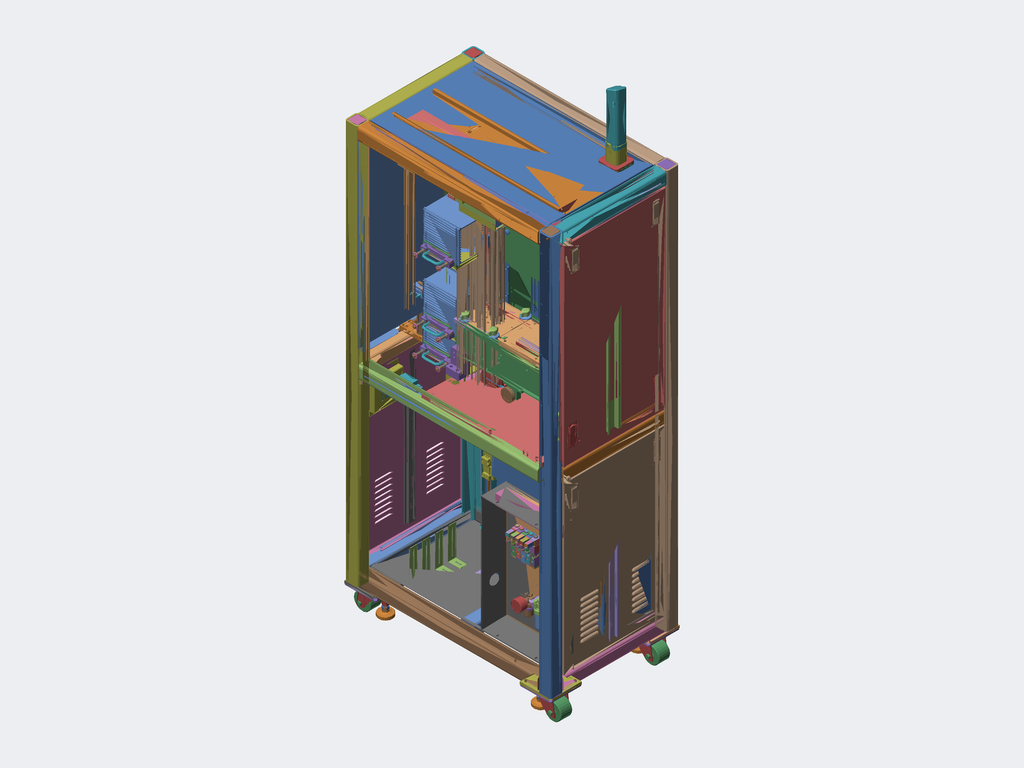Assembly | STEP file | 160 different items | 302 placed
Parts list (item | name | quantity | parent item | size | volume):
1 | 138-90 material plate | x1 | in FBDS-CS | - | -
2 | - | x1 | - | 63 x 161.8 x 74.5 mm | 210839 mm3
3 | - | x1 | in FYTH14-L05-650-BC-M40-C4^FBDS-SJ | 62.422 x 99.9 x 129.5 mm | 546623 mm3
4 | 42CME02^FBDS-CS | x1 | in FBDS-CS | - | 53634 mm3
5 | 508 material box | x3 | in FBDS-SJ | - | -
6 | 5X18 flat washer | x6 | in FBDS-XLYJ | - | -
7 | 6701ZZ | x3 | in FBDS-CS | 18 x 18 x 4 mm | 565.487 mm3
8 | AC20001 | x1 | in FB-DS-PQ | 86 x 133.8 x 136 mm | 222046 mm3
9 | - | x1 | - | 63 x 130 x 63 mm | 202293 mm3
10 | - | x1 | - | 54 x 3 x 31 mm | 4823 mm3
11 | - | x1 | - | 73 x 64.5 x 64.5 mm | 159497 mm3
12 | - | x1 | - | 64.5 x 64.5 x 62 mm | 97512 mm3
13 | - | x1 | - | 42 x 64.5 x 64.5 mm | 111603 mm3
14 | - | x2 | - | 16 x 16 x 95 mm | 18202 mm3
15 | - | x1 | - | 135 x 73 x 48 mm | 191196 mm3
16 | - | x1 | - | 45 x 29 x 29 mm | 22988 mm3
17 | - | x1 | - | 127 x 40 x 12 mm | 55019 mm3
18 | - | x1 | - | 75 x 75 x 14 mm | 44712 mm3
19 | AP-DJ2711 outline drawing | x1 | in DLZFJZJ | - | -
20 | Air distribution-cable trough | x1 | in FB-DS-PQ | - | -
21 | C-MLG12-270 | x1 | in MGN12C2R270Z0CM | 12 x 8 x 270 mm | 22993 mm3
22 | C-MLGB12 | x2 | in MGN12C2R270Z0CM | 27 x 10 x 35.3 mm | 6611 mm3
23 | C-TBCR-S3M100.stp | x1 | in FBDS-CS | 21 x 25 x 4 mm | 1633 mm3
24 | C-VUR8-25 | x6 | in FBDS-XLYJ | 9.3 x 25 x 9.325 mm | 430.371 mm3
25 | CS-DS-001 | x1 | in FB-DS | 640 x 460 x 225 mm | 1382165 mm3
26 | CS-DS-002 | x1 | in FB-DS | 615 x 440 x 12 mm | 579701 mm3
27 | CS-DS-003 | x1 | in FB-DS-PQ | 430 x 240 x 12 mm | 228512 mm3
28 | CS-DS-004 | x1 | in FB-DS-PQ | 450 x 260 x 140 mm | 518743 mm3
29 | C_C04_N01 | x2 | in FBDS-CS | 125 x 4.01 x 4 mm | 907.682 mm3
30 | Cable trough | x1 | in FB-DS | - | -
31 | Changxin changeover switch LW26-20 | x1 | in ZHKGZJ | - | -
32 | Compression lever-type surface lock XAT31 | x8 | in HSCBZJ, HXCBZJ, YSCBZJ, YXCBZJ | - | -
33 | Compression locking adjustable surface lock XAT85-B | x4 | in HSCBZJ, YSCBZJ | - | -
34 | Copy EGH15C_left cover_temp^EGH15CA2R240Z0C | x2 | in EGH15CA2R240Z0C | - | -
35 | Copy EGH15C_right cover_temp^EGH15CA2R240Z0C | x2 | in EGH15CA2R240Z0C | - | -
36 | Copy M4H^EGH15CA2R240Z0C | x4 | in EGH15CA2R240Z0C | - | -
37 | DS-HJ_default<machined> | x1 | in FBDS | - | -
38 | DSJIN1 | x1 | in FBDS-SJ | 22 x 400 x 10 mm | 85812 mm3
39 | DSJIN2 | x1 | in FBDS-SJ | 30 x 400 x 10 mm | 118112 mm3
40 | Door catch body | x2 | in Door catch | - | -
41 | Door catch magnet | x2 | in Door catch | - | -
42 | EE-SX672NPN^FYTH14-L05-650-BC-M40-C4_FBDS-SJ | x3 | in FYTH14-L05-650-BC-M40-C4^FBDS-SJ | 26 x 39 x 13.7 mm | 3424 mm3
43 | EGH15CA2R600Z0C | x2 | in EGH15CA2R240Z0C | 15 x 12.5 x 240 mm | 38381 mm3
44 | FBDS-BEI | x1 | in FBDS | 370 x 156 x 10 mm | 569992 mm3
45 | FBDS-BJ-001 | x1 | in ZXCBZJ | 398 x 648 x 31 mm | 500779 mm3
46 | FBDS-BJ-002 | x1 | in YXCBZJ | 396 x 651 x 31 mm | 529304 mm3
47 | FBDS-BJ-003 | x1 | in FBDS | 398 x 748 x 25 mm | 585293 mm3
48 | FBDS-BJ-004 | x1 | in HXCBZJ | 695 x 650 x 31 mm | 909135 mm3
49 | FBDS-BJ-006 | x1 | in HSCBZJ | 696 x 746 x 20 mm | 1021844 mm3
50 | FBDS-BJ-007 | x1 | in DGZJ | 698 x 398 x 20 mm | 721973 mm3
51 | FBDS-BJ-008 | x1 | in YSCBZJ | 396 x 746 x 20 mm | 589557 mm3
52 | FBDS-BJ-012 | x1 | in DLZFJZJ | 237 x 60 x 40 mm | 29907 mm3
53 | FBDS-BJ-014 | x4 | in FBDS | 20 x 85 x 15 mm | 4798 mm3
54 | FBDS-BJ-015 | x1 | in FBDS | 27 x 32 x 60 mm | 6673 mm3
55 | FBDS-BJ-016 | x1 | in DLZFJZJ | 160 x 60 x 25 mm | 23506 mm3
56 | FBDS-BJ-017 | x1 | in ZHKGZJ | 113.4 x 140.4 x 20 mm | 34877 mm3
57 | FBDS-BJ-021 | x1 | in FBDS | 115 x 11.5 x 24.473 mm | 6686 mm3
58 | FBDS-BJ-023 | x4 | in FBDS | 46.5 x 121.5 x 30 mm | 6584 mm3
59 | FBDS-BJ-024 | x1 | in FBDS | 25 x 10 x 1.5 mm | 311.948 mm3
60 | FBDS-CS-001 | x1 | in FBDS-CS | 60 x 19.5 x 8 mm | 8486 mm3
61 | FBDS-CS-002 | x1 | in FBDS-CS | 42.5 x 27 x 21 mm | 8750 mm3
62 | FBDS-CS-003 | x1 | in FBDS-CS | 100 x 60 x 11.5 mm | 64777 mm3
63 | FBDS-CS-004 | x1 | in FBDS-CS | 279.5 x 130 x 130 mm | 91348 mm3
64 | FBDS-CS-005 | x1 | in FBDS-CS | 31.5 x 10 x 36.5 mm | 1072 mm3
65 | FBDS-CS-006 | x2 | in FBDS-CS | 45 x 17 x 2 mm | 1395 mm3
66 | FBDS-CS-007 | x1 | in FBDS-CS | 159 x 11 x 32 mm | 45788 mm3
67 | FBDS-CS-008 | x1 | in FBDS-CS | 159 x 11 x 32 mm | 45787 mm3
68 | FBDS-CS-009 | x1 | in FBDS-CS | 34 x 11 x 9 mm | 2531 mm3
69 | FBDS-CS-010 | x2 | in FBDS-CS | 5 x 5 x 14.5 mm | 281.042 mm3
70 | FBDS-CS-011 | x2 | in FBDS-CS | 50 x 80 x 45 mm | 112378 mm3
71 | FBDS-CS-012 | x2 | in FBDS-CS | 290 x 50 x 20 mm | 283331 mm3
72 | FBDS-CS-013 | x2 | in FBDS-CS | 38 x 50 x 95 mm | 75969 mm3
73 | FBDS-CS-014 | x1 | in FBDS-CS | 30 x 88 x 84 mm | 6954 mm3
74 | FBDS-CS-015 | x1 | in FBDS-CS | 33 x 30 x 8 mm | 5456 mm3
75 | FBDS-CS-016 | x2 | in FBDS-CS | 70 x 30 x 8 mm | 11291 mm3
76 | FBDS-CS-017 | x1 | in FBDS-CS | 60 x 64 x 8 mm | 17841 mm3
77 | FBDS-CS-018 | x1 | in FBDS-CS | 72 x 40 x 15 mm | 21999 mm3
78 | FBDS-CS-019 | x1 | in FBDS-CS | 50 x 33.5 x 50 mm | 22855 mm3
79 | FBDS-CS-020 | x1 | in FBDS-CS | 22 x 26 x 6 mm | 2342 mm3
80 | FBDS-CS-021 | x1 | in FBDS-CS | 45 x 45 x 16 mm | 16300 mm3
81 | FBDS-CS-022 | x1 | in FBDS-CS | 280 x 74 x 10 mm | 161210 mm3
82 | FBDS-CS-023 | x1 | in FBDS-CS | 218 x 27 x 10 mm | 50909 mm3
83 | FBDS-CS-024 | x1 | in FBDS-CS | 20 x 14 x 8 mm | 1034 mm3
84 | FBDS-CS-025 | x1 | in FBDS-CS | 20 x 14 x 8.5 mm | 1206 mm3
85 | FBDS-CS-026 | x1 | in FBDS-CS | 146 x 140 x 10 mm | 153176 mm3
86 | FBDS-CS-027 | x1 | in FBDS-CS | 40 x 70 x 10 mm | 7093 mm3
87 | FBDS-CS-028 | x1 | in FBDS-CS | 136 x 76 x 18 mm | 111682 mm3
88 | FBDS-CS-029 | x1 | in FBDS-CS | 136 x 76 x 22 mm | 100751 mm3
89 | FBDS-CS-030 | x1 | in FBDS-CS | 438 x 110 x 15 mm | 713481 mm3
90 | FBDS-CS-031 | x1 | in FBDS-CS | 438 x 110 x 15 mm | 703855 mm3
91 | FBDS-CS-032 | x1 | in FBDS-CS | 11 x 11 x 32 mm | 1542 mm3
92 | FBDS-CS-034 | x1 | in FBDS-CS | 32 x 41.5 x 18 mm | 2551 mm3
93 | FBDS-CS-035 | x1 | in FBDS-CS | 35 x 15 x 9 mm | 3093 mm3
94 | FBDS-JIN | x1 | in FBDS | 124 x 260 x 10 mm | 178303 mm3
95 | FBDS-TB | x1 | in FBDS | 669.5 x 475 x 12 mm | 2998204 mm3
96 | FBDS-TL-001 | x1 | in FBDS-TL | 8 x 173.5 x 50 mm | 68338 mm3
97 | FBDS-TL-002 | x1 | in FBDS-TL | 10 x 10 x 20 mm | 1243 mm3
98 | FBDS-TL-003 | x1 | in FBDS-TL | 22 x 40 x 5 mm | 2172 mm3
99 | FBDS-TL-004 | x1 | in FBDS | 113 x 40 x 15 mm | 62186 mm3
100 | FBDS-TL-005 | x1 | in FBDS-TL | 25 x 36.5 x 22 mm | 1956 mm3
101 | FBDS-TL-006 | x1 | in FBDS-TL | 26 x 40 x 8 mm | 5029 mm3
102 | FBDS-ZUO | x1 | in FBDS | 136 x 124 x 10 mm | 164198 mm3
103 | G_ST70_XX_03818V(1) | x1 | in FB-DS | - | -
104 | High-current double-layer terminal block | x20 | in FB-DS | - | -
105 | JAJ-65_adjusters | x4 | in JAJ-65 | 53 x 65 x 53 mm | 36497 mm3
106 | JAJ-65_base | x4 | in JAJ-65 | 97.399 x 74 x 67.001 mm | 43204 mm3
107 | JAJ-65_caster | x4 | in JAJ-65 | 65 x 65 x 74 mm | 148221 mm3
108 | JAJ-65_plate | x4 | in JAJ-65 | 120 x 16 x 120 mm | 79899 mm3
109 | JAJ_SLMNA-M12 | x4 | in JAJ-65 | 19 x 10 x 21.939 mm | 2279 mm3
110 | JIN-1 | x1 | in FBDS | 124 x 260 x 10 mm | 178303 mm3
111 | Jingjiake BBX-441 | x2 | in FBDS-CS, FBDS-TL | - | -
112 | KRBT-S3M-100- 179 | x1 | in FBDS-CS | 27.07 x 256.613 x 10 mm | 8091 mm3
113 | LED light | x1 | in FBDS | - | -
114 | - | x2 | - | 37 x 48 x 48 mm | 17828 mm3
115 | LMUF8G | x6 | in FBDS-XLYJ | 24 x 15 x 15 mm | 2996 mm3
116 | LY2N - J _ DTF-08A ( PTF-08A )-1.step | x5 | in FB-DS | 73.5 x 65 x 23.1 mm | 52348 mm3
117 | MBDLN25SE | x1 | in FB-DS | 58.866 x 180 x 153.541 mm | 995298 mm3
118 | MGJ10-20-F8B_BODY | x1 | in MGJ10-20-F8BL(0_0) | 39 x 33 x 17 mm | 15219 mm3
119 | MGJ10-20-F8B_CYROD | x1 | in MGJ10-20-F8BL(0_0) | 37 x 32 x 10 mm | 3940 mm3
120 | MGJ_D-F8B | x2 | in MGJ10-20-F8BL(0_0) | 10 x 23 x 4.6 mm | 489.26 mm3
121 | MHZ2-6D2_Body(0).stp | x1 | in MHZ2-6D2-M9BAL | 20 x 10 x 38.8 mm | 6543 mm3
122 | MHZ2-6D2_Finger(0).stp | x2 | in MHZ2-6D2-M9BAL | 8.55 x 5 x 17.2 mm | 286.489 mm3
123 | - | x1 | in MKB16_10LZ_0_0_ | 16 x 16 x 60 mm | 4417 mm3
124 | - | x1 | in MKB16_10LZ_0_0_ | 29 x 29 x 65 mm | 26524 mm3
125 | NXBLE-32 2P C20 30MA 6KA | x1 | in FB-DS | 93.6 x 75.273 x 71.5 mm | 301001 mm3
126 | PMD1212PMB1-A (2).GN | x2 | in FBDS | - | -
127 | PSSGGZ8-50-F7-B5-P4-N5-SC10 | x6 | in FBDS-XLYJ | 57 x 8 x 8 mm | 2360 mm3
128 | Protective wire ring ID 35mm | x4 | in FB-DS, FB-DS-PQ | - | -
129 | Protective wire ring ID 60mm | x1 | in FB-DS | - | -
130 | Proximity switch | x1 | in FBDS | - | -
131 | QCTHA0834-14_01^qctha0834-14_FBDS-CS | x4 | in qctha0834-14^FBDS-CS | 34 x 29 x 34 mm | 9325 mm3
132 | QCTHA0834-14_02^qctha0834-14_FBDS-CS | x4 | in qctha0834-14^FBDS-CS | 34 x 43.5 x 22 mm | 5217 mm3
133 | QCTHA0834-14_03^qctha0834-14_FBDS-CS | x4 | in qctha0834-14^FBDS-CS | 5.5 x 5.5 x 9 mm | 105.567 mm3
134 | QCTHA0834-14_04^qctha0834-14_FBDS-CS | x4 | in qctha0834-14^FBDS-CS | 5.5 x 5.5 x 9 mm | 105.567 mm3
135 | QCTHA0834-14_05^qctha0834-14_FBDS-CS | x4 | in qctha0834-14^FBDS-CS | 5.5 x 5.5 x 9 mm | 105.567 mm3
136 | SD-350 | x2 | in FB-DS | - | -
137 | - | x1 | in FYTH14-L05-650-BC-M40-C4^FBDS-SJ | 135 x 74.2 x 900.5 mm | 2232151 mm3
138 | - | x1 | in FYTH14-L05-650-BC-M40-C4^FBDS-SJ | 133 x 31.5 x 140 mm | 288957 mm3
139 | - | x1 | in FYTH14-L05-650-BC-M40-C4^FBDS-SJ | 8 x 30 x 70 mm | 1347 mm3
140 | TAAS3M-26-100-P5 | x1 | in FBDS-CS | 15 x 28 x 28 mm | 6135 mm3
141 | TAAS3M_26_100_P8 | x1 | in FBDS-CS | 15 x 28 x 28 mm | 5701 mm3
142 | TWD15-C15-R28-12(S0)_cable | x1 | in TWD15-C15-R28-12(S0) | 206.68 x 96 x 25 mm | 76610 mm3
143 | TWD15-C15-R28-3_fix | x1 | in TWD15-C15-R28-12(S0) | 40 x 20 x 24 mm | 4424 mm3
144 | TWD15-C15-R28-3_free | x1 | in TWD15-C15-R28-12(S0) | 39.871 x 19.871 x 24.8 mm | 3618 mm3
145 | Three-color signal light 5i-i7 | x1 | in DGZJ | - | -
146 | User Library-4V110 Pneumatic solenoid valve | x1 | in FB-DS-PQ | - | -
147 | XL-003 | x3 | in FBDS-XLYJ | 69 x 19 x 15 mm | 19058 mm3
148 | XL-004 | x3 | in FBDS-XLYJ | 125 x 30 x 8 mm | 16770 mm3
149 | XL-005 | x3 | in FBDS-XLYJ | 110 x 22 x 20 mm | 25117 mm3
150 | XL-007 | x3 | in FBDS-XLYJ | 68 x 34 x 8 mm | 5416 mm3
151 | XL-008 | x3 | in FBDS-XLYJ | 108 x 125 x 8 mm | 107538 mm3
152 | XL-01 | x1 | in FBDS-SJ | 148 x 600 x 16 mm | 970586 mm3
153 | c45-150 | x2 | in FB-DS | 7.5 x 150 x 35 mm | 6844 mm3
154 | c45-310 | x1 | in FB-DS | 7.5 x 310 x 35 mm | 14144 mm3
155 | cjx2_d18.step | x1 | in FB-DS | 46 x 86.1 x 80 mm | 227917 mm3
156 | cl57 | x2 | in FB-DS | 116 x 26.5 x 69.2 mm | 66136 mm3
157 | hexagon socket head cap screws gb_GB_FASTENER_SCREWS_HSHCS M5X8-C | x6 | in FBDS-XLYJ | 13 x 8.5 x 8.5 mm | 398.856 mm3
158 | pm-y45 | x2 | in FBDS-CS | 72.1 x 14.6 x 13.4 mm | 1769 mm3
159 | screw_STEP.stp | x1 | in R16-5T3-FSI-100-100-0.05.stp | 130 x 16 x 16 mm | 22700 mm3
160 | - | x4 | in EGH15CA2R240Z0C | - | -